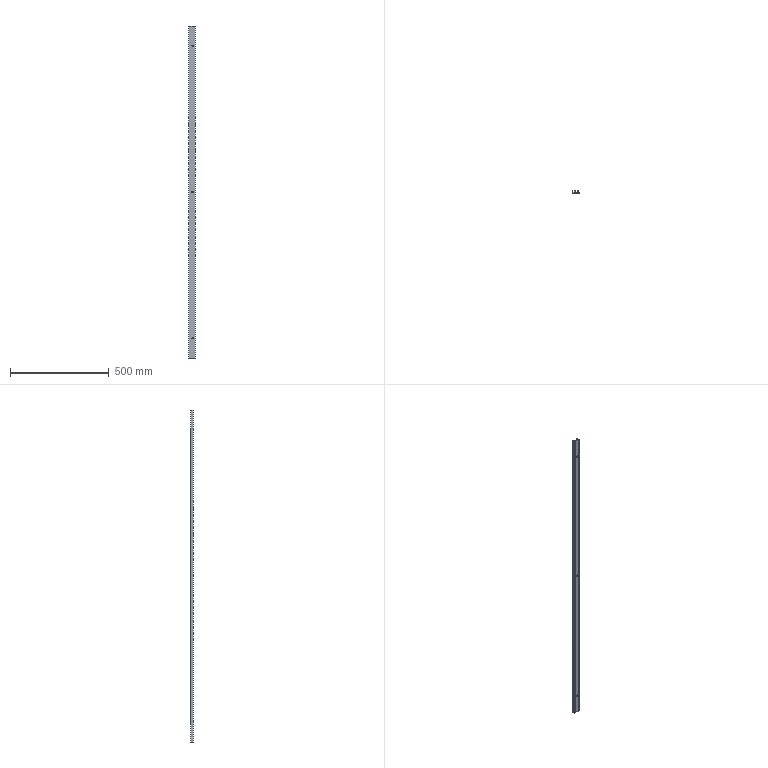Part | 1 solid | 31 faces | box 33.5 x 13.5 x 1682 mm | volume 314894 mm3 | plane 16 | cylinder 9 | cone 6 | commonest cylinder face diameters 2 x3 13.44 x3 4 x2 1.5 x1
STEP:
#1=CARTESIAN_POINT('',(20.,0.,1485.72));
#2=VERTEX_POINT('',#1);
#3=CARTESIAN_POINT('',(20.,0.,1478.28));
#4=VERTEX_POINT('',#3);
#5=CARTESIAN_POINT('',(20.,0.,1482.));
#6=DIRECTION('',(0.,-1.,0.));
#7=DIRECTION('',(0.,0.,-1.));
#8=AXIS2_PLACEMENT_3D('',#5,#6,#7);
#9=CIRCLE('',#8,3.72);
#10=EDGE_CURVE('',#2,#4,#9,.T.);
#11=ORIENTED_EDGE('',*,*,#10,.T.);
#12=CARTESIAN_POINT('',(20.,3.,1475.28));
#13=VERTEX_POINT('',#12);
#14=CARTESIAN_POINT('',(20.,3.,1475.28));
#15=DIRECTION('',(0.,0.7071,-0.7071));
#16=VECTOR('',#15,1000.);
#17=LINE('',#14,#16);
#18=EDGE_CURVE('',#4,#13,#17,.T.);
#19=ORIENTED_EDGE('',*,*,#18,.T.);
#20=CARTESIAN_POINT('',(20.,3.,1488.72));
#21=VERTEX_POINT('',#20);
#22=CARTESIAN_POINT('',(20.,3.,1482.));
#23=DIRECTION('',(0.,1.,0.));
#24=DIRECTION('',(0.,0.,1.));
#25=AXIS2_PLACEMENT_3D('',#22,#23,#24);
#26=CIRCLE('',#25,6.72);
#27=EDGE_CURVE('',#13,#21,#26,.T.);
#28=ORIENTED_EDGE('',*,*,#27,.T.);
#29=CARTESIAN_POINT('',(20.,3.,1488.72));
#30=DIRECTION('',(0.,0.7071,0.7071));
#31=VECTOR('',#30,1000.);
#32=LINE('',#29,#31);
#33=EDGE_CURVE('',#2,#21,#32,.T.);
#34=ORIENTED_EDGE('',*,*,#33,.F.);
#35=EDGE_LOOP('',(#11,#19,#28,#34));
#36=FACE_OUTER_BOUND('',#35,.T.);
#37=CARTESIAN_POINT('',(20.,3.,1482.));
#38=DIRECTION('',(0.,1.,0.));
#39=DIRECTION('',(0.,0.,1.));
#40=AXIS2_PLACEMENT_3D('',#37,#38,#39);
#41=CONICAL_SURFACE('',#40,6.72,0.7854);
#42=ADVANCED_FACE('',(#36),#41,.F.);
#43=CARTESIAN_POINT('',(20.,0.,3.72));
#44=VERTEX_POINT('',#43);
#45=CARTESIAN_POINT('',(20.,0.,-3.72));
#46=VERTEX_POINT('',#45);
#47=CARTESIAN_POINT('',(20.,0.,0.));
#48=DIRECTION('',(0.,-1.,0.));
#49=DIRECTION('',(0.,0.,-1.));
#50=AXIS2_PLACEMENT_3D('',#47,#48,#49);
#51=CIRCLE('',#50,3.72);
#52=EDGE_CURVE('',#44,#46,#51,.T.);
#53=ORIENTED_EDGE('',*,*,#52,.T.);
#54=CARTESIAN_POINT('',(20.,3.,-6.72));
#55=VERTEX_POINT('',#54);
#56=CARTESIAN_POINT('',(20.,3.,-6.72));
#57=DIRECTION('',(0.,0.7071,-0.7071));
#58=VECTOR('',#57,1000.);
#59=LINE('',#56,#58);
#60=EDGE_CURVE('',#46,#55,#59,.T.);
#61=ORIENTED_EDGE('',*,*,#60,.T.);
#62=CARTESIAN_POINT('',(20.,3.,6.72));
#63=VERTEX_POINT('',#62);
#64=CARTESIAN_POINT('',(20.,3.,0.));
#65=DIRECTION('',(0.,1.,0.));
#66=DIRECTION('',(0.,0.,1.));
#67=AXIS2_PLACEMENT_3D('',#64,#65,#66);
#68=CIRCLE('',#67,6.72);
#69=EDGE_CURVE('',#55,#63,#68,.T.);
#70=ORIENTED_EDGE('',*,*,#69,.T.);
#71=CARTESIAN_POINT('',(20.,3.,6.72));
#72=DIRECTION('',(0.,0.7071,0.7071));
#73=VECTOR('',#72,1000.);
#74=LINE('',#71,#73);
#75=EDGE_CURVE('',#44,#63,#74,.T.);
#76=ORIENTED_EDGE('',*,*,#75,.F.);
#77=EDGE_LOOP('',(#53,#61,#70,#76));
#78=FACE_OUTER_BOUND('',#77,.T.);
#79=CARTESIAN_POINT('',(20.,3.,0.));
#80=DIRECTION('',(0.,1.,0.));
#81=DIRECTION('',(0.,0.,1.));
#82=AXIS2_PLACEMENT_3D('',#79,#80,#81);
#83=CONICAL_SURFACE('',#82,6.72,0.7854);
#84=ADVANCED_FACE('',(#78),#83,.F.);
#85=CARTESIAN_POINT('',(20.,0.,744.72));
#86=VERTEX_POINT('',#85);
#87=CARTESIAN_POINT('',(20.,0.,737.28));
#88=VERTEX_POINT('',#87);
#89=CARTESIAN_POINT('',(20.,0.,741.));
#90=DIRECTION('',(0.,-1.,0.));
#91=DIRECTION('',(0.,0.,-1.));
#92=AXIS2_PLACEMENT_3D('',#89,#90,#91);
#93=CIRCLE('',#92,3.72);
#94=EDGE_CURVE('',#86,#88,#93,.T.);
#95=ORIENTED_EDGE('',*,*,#94,.T.);
#96=CARTESIAN_POINT('',(20.,3.,734.28));
#97=VERTEX_POINT('',#96);
#98=CARTESIAN_POINT('',(20.,3.,734.28));
#99=DIRECTION('',(0.,0.7071,-0.7071));
#100=VECTOR('',#99,1000.);
#101=LINE('',#98,#100);
#102=EDGE_CURVE('',#88,#97,#101,.T.);
#103=ORIENTED_EDGE('',*,*,#102,.T.);
#104=CARTESIAN_POINT('',(20.,3.,747.72));
#105=VERTEX_POINT('',#104);
#106=CARTESIAN_POINT('',(20.,3.,741.));
#107=DIRECTION('',(0.,1.,0.));
#108=DIRECTION('',(0.,0.,1.));
#109=AXIS2_PLACEMENT_3D('',#106,#107,#108);
#110=CIRCLE('',#109,6.72);
#111=EDGE_CURVE('',#97,#105,#110,.T.);
#112=ORIENTED_EDGE('',*,*,#111,.T.);
#113=CARTESIAN_POINT('',(20.,3.,747.72));
#114=DIRECTION('',(0.,0.7071,0.7071));
#115=VECTOR('',#114,1000.);
#116=LINE('',#113,#115);
#117=EDGE_CURVE('',#86,#105,#116,.T.);
#118=ORIENTED_EDGE('',*,*,#117,.F.);
#119=EDGE_LOOP('',(#95,#103,#112,#118));
#120=FACE_OUTER_BOUND('',#119,.T.);
#121=CARTESIAN_POINT('',(20.,3.,741.));
#122=DIRECTION('',(0.,1.,0.));
#123=DIRECTION('',(0.,0.,1.));
#124=AXIS2_PLACEMENT_3D('',#121,#122,#123);
#125=CONICAL_SURFACE('',#124,6.72,0.7854);
#126=ADVANCED_FACE('',(#120),#125,.F.);
#127=CARTESIAN_POINT('',(24.5,10.5,-4.991));
#128=VERTEX_POINT('',#127);
#129=CARTESIAN_POINT('',(24.5,10.5,-100.));
#130=VERTEX_POINT('',#129);
#131=CARTESIAN_POINT('',(24.5,10.5,-100.));
#132=DIRECTION('',(0.,0.,-1.));
#133=VECTOR('',#132,1000.);
#134=LINE('',#131,#133);
#135=EDGE_CURVE('',#128,#130,#134,.T.);
#136=ORIENTED_EDGE('',*,*,#135,.F.);
#137=CARTESIAN_POINT('',(24.5,10.5,4.991));
#138=VERTEX_POINT('',#137);
#139=CARTESIAN_POINT('',(24.5,10.5,-4.991));
#140=CARTESIAN_POINT('',(24.5,10.638,-4.991));
#141=CARTESIAN_POINT('',(24.515,10.777,-4.978));
#142=CARTESIAN_POINT('',(24.57,11.043,-4.927));
#143=CARTESIAN_POINT('',(24.611,11.171,-4.889));
#144=CARTESIAN_POINT('',(24.765,11.529,-4.74));
#145=CARTESIAN_POINT('',(24.907,11.728,-4.597));
#146=CARTESIAN_POINT('',(25.205,12.04,-4.256));
#147=CARTESIAN_POINT('',(25.365,12.156,-4.055));
#148=CARTESIAN_POINT('',(25.663,12.325,-3.627));
#149=CARTESIAN_POINT('',(25.806,12.38,-3.395));
#150=CARTESIAN_POINT('',(26.19,12.494,-2.672));
#151=CARTESIAN_POINT('',(26.387,12.501,-2.161));
#152=CARTESIAN_POINT('',(26.654,12.499,-1.091));
#153=CARTESIAN_POINT('',(26.72,12.488,-0.5481));
#154=CARTESIAN_POINT('',(26.72,12.488,0.2773));
#155=CARTESIAN_POINT('',(26.703,12.49,0.5529));
#156=CARTESIAN_POINT('',(26.636,12.496,1.095));
#157=CARTESIAN_POINT('',(26.586,12.499,1.362));
#158=CARTESIAN_POINT('',(26.388,12.501,2.155));
#159=CARTESIAN_POINT('',(26.188,12.493,2.677));
#160=CARTESIAN_POINT('',(25.805,12.38,3.396));
#161=CARTESIAN_POINT('',(25.662,12.324,3.629));
#162=CARTESIAN_POINT('',(25.438,12.197,3.95));
#163=CARTESIAN_POINT('',(25.362,12.147,4.053));
#164=CARTESIAN_POINT('',(25.208,12.03,4.249));
#165=CARTESIAN_POINT('',(25.13,11.961,4.342));
#166=CARTESIAN_POINT('',(24.98,11.805,4.513));
#167=CARTESIAN_POINT('',(24.908,11.717,4.591));
#168=CARTESIAN_POINT('',(24.774,11.518,4.73));
#169=CARTESIAN_POINT('',(24.714,11.408,4.79));
#170=CARTESIAN_POINT('',(24.612,11.172,4.888));
#171=CARTESIAN_POINT('',(24.57,11.043,4.927));
#172=CARTESIAN_POINT('',(24.515,10.778,4.978));
#173=CARTESIAN_POINT('',(24.5,10.64,4.991));
#174=CARTESIAN_POINT('',(24.5,10.5,4.991));
#175=B_SPLINE_CURVE_WITH_KNOTS('',3,(#139,#140,#141,#142,#143,#144,#145,#146,#147,#148,#149,#150,#151,#152,#153,#154,#155,#156,#157,#158,#159,#160,#161,#162,#163,#164,#165,#166,#167,#168,#169,#170,#171,#172,#173,#174),.UNSPECIFIED.,.F.,.F.,(4,2,2,2,2,2,2,2,2,2,2,2,2,2,2,2,2,4),(0.01321,0.01362,0.01403,0.01486,0.01569,0.01651,0.01816,0.01981,0.02064,0.02146,0.02311,0.02394,0.02435,0.02477,0.02518,0.02559,0.026,0.02642),.UNSPECIFIED.);
#176=EDGE_CURVE('',#128,#138,#175,.T.);
#177=ORIENTED_EDGE('',*,*,#176,.T.);
#178=CARTESIAN_POINT('',(24.5,10.5,736.009));
#179=VERTEX_POINT('',#178);
#180=CARTESIAN_POINT('',(24.5,10.5,-100.));
#181=DIRECTION('',(0.,0.,-1.));
#182=VECTOR('',#181,1000.);
#183=LINE('',#180,#182);
#184=EDGE_CURVE('',#179,#138,#183,.T.);
#185=ORIENTED_EDGE('',*,*,#184,.F.);
#186=CARTESIAN_POINT('',(24.5,10.5,745.991));
#187=VERTEX_POINT('',#186);
#188=CARTESIAN_POINT('',(24.5,10.5,736.009));
#189=CARTESIAN_POINT('',(24.5,10.638,736.009));
#190=CARTESIAN_POINT('',(24.515,10.777,736.022));
#191=CARTESIAN_POINT('',(24.57,11.043,736.073));
#192=CARTESIAN_POINT('',(24.611,11.171,736.111));
#193=CARTESIAN_POINT('',(24.765,11.529,736.26));
#194=CARTESIAN_POINT('',(24.907,11.728,736.403));
#195=CARTESIAN_POINT('',(25.205,12.04,736.744));
#196=CARTESIAN_POINT('',(25.365,12.156,736.945));
#197=CARTESIAN_POINT('',(25.663,12.325,737.373));
#198=CARTESIAN_POINT('',(25.806,12.38,737.605));
#199=CARTESIAN_POINT('',(26.19,12.494,738.328));
#200=CARTESIAN_POINT('',(26.387,12.501,738.839));
#201=CARTESIAN_POINT('',(26.654,12.499,739.909));
#202=CARTESIAN_POINT('',(26.72,12.488,740.452));
#203=CARTESIAN_POINT('',(26.72,12.488,741.277));
#204=CARTESIAN_POINT('',(26.703,12.49,741.553));
#205=CARTESIAN_POINT('',(26.636,12.496,742.095));
#206=CARTESIAN_POINT('',(26.586,12.499,742.362));
#207=CARTESIAN_POINT('',(26.388,12.501,743.155));
#208=CARTESIAN_POINT('',(26.188,12.493,743.677));
#209=CARTESIAN_POINT('',(25.805,12.38,744.396));
#210=CARTESIAN_POINT('',(25.662,12.324,744.629));
#211=CARTESIAN_POINT('',(25.438,12.197,744.95));
#212=CARTESIAN_POINT('',(25.362,12.147,745.053));
#213=CARTESIAN_POINT('',(25.208,12.03,745.249));
#214=CARTESIAN_POINT('',(25.13,11.961,745.342));
#215=CARTESIAN_POINT('',(24.98,11.805,745.513));
#216=CARTESIAN_POINT('',(24.908,11.717,745.591));
#217=CARTESIAN_POINT('',(24.774,11.518,745.73));
#218=CARTESIAN_POINT('',(24.714,11.408,745.79));
#219=CARTESIAN_POINT('',(24.612,11.172,745.888));
#220=CARTESIAN_POINT('',(24.57,11.043,745.927));
#221=CARTESIAN_POINT('',(24.515,10.778,745.978));
#222=CARTESIAN_POINT('',(24.5,10.64,745.991));
#223=CARTESIAN_POINT('',(24.5,10.5,745.991));
#224=B_SPLINE_CURVE_WITH_KNOTS('',3,(#188,#189,#190,#191,#192,#193,#194,#195,#196,#197,#198,#199,#200,#201,#202,#203,#204,#205,#206,#207,#208,#209,#210,#211,#212,#213,#214,#215,#216,#217,#218,#219,#220,#221,#222,#223),.UNSPECIFIED.,.F.,.F.,(4,2,2,2,2,2,2,2,2,2,2,2,2,2,2,2,2,4),(0.01321,0.01362,0.01403,0.01486,0.01569,0.01651,0.01816,0.01981,0.02064,0.02146,0.02311,0.02394,0.02435,0.02477,0.02518,0.02559,0.026,0.02642),.UNSPECIFIED.);
#225=EDGE_CURVE('',#179,#187,#224,.T.);
#226=ORIENTED_EDGE('',*,*,#225,.T.);
#227=CARTESIAN_POINT('',(24.5,10.5,1477.009));
#228=VERTEX_POINT('',#227);
#229=CARTESIAN_POINT('',(24.5,10.5,-100.));
#230=DIRECTION('',(0.,0.,-1.));
#231=VECTOR('',#230,1000.);
#232=LINE('',#229,#231);
#233=EDGE_CURVE('',#228,#187,#232,.T.);
#234=ORIENTED_EDGE('',*,*,#233,.F.);
#235=CARTESIAN_POINT('',(24.5,10.5,1486.991));
#236=VERTEX_POINT('',#235);
#237=CARTESIAN_POINT('',(24.5,10.5,1477.009));
#238=CARTESIAN_POINT('',(24.5,10.64,1477.009));
#239=CARTESIAN_POINT('',(24.514,10.776,1477.022));
#240=CARTESIAN_POINT('',(24.57,11.042,1477.073));
#241=CARTESIAN_POINT('',(24.611,11.171,1477.111));
#242=CARTESIAN_POINT('',(24.713,11.408,1477.209));
#243=CARTESIAN_POINT('',(24.775,11.519,1477.27));
#244=CARTESIAN_POINT('',(24.908,11.717,1477.409));
#245=CARTESIAN_POINT('',(24.981,11.806,1477.488));
#246=CARTESIAN_POINT('',(25.207,12.042,1477.746));
#247=CARTESIAN_POINT('',(25.363,12.155,1477.942));
#248=CARTESIAN_POINT('',(25.665,12.326,1478.376));
#249=CARTESIAN_POINT('',(25.806,12.38,1478.605));
#250=CARTESIAN_POINT('',(26.061,12.456,1479.084));
#251=CARTESIAN_POINT('',(26.176,12.476,1479.337));
#252=CARTESIAN_POINT('',(26.372,12.498,1479.849));
#253=CARTESIAN_POINT('',(26.454,12.501,1480.109));
#254=CARTESIAN_POINT('',(26.586,12.499,1480.638));
#255=CARTESIAN_POINT('',(26.636,12.496,1480.907));
#256=CARTESIAN_POINT('',(26.703,12.49,1481.453));
#257=CARTESIAN_POINT('',(26.72,12.488,1481.729));
#258=CARTESIAN_POINT('',(26.72,12.488,1482.275));
#259=CARTESIAN_POINT('',(26.703,12.49,1482.547));
#260=CARTESIAN_POINT('',(26.637,12.496,1483.089));
#261=CARTESIAN_POINT('',(26.587,12.499,1483.36));
#262=CARTESIAN_POINT('',(26.387,12.501,1484.161));
#263=CARTESIAN_POINT('',(26.191,12.494,1484.671));
#264=CARTESIAN_POINT('',(25.805,12.38,1485.396));
#265=CARTESIAN_POINT('',(25.663,12.325,1485.627));
#266=CARTESIAN_POINT('',(25.364,12.155,1486.057));
#267=CARTESIAN_POINT('',(25.205,12.039,1486.256));
#268=CARTESIAN_POINT('',(24.981,11.805,1486.512));
#269=CARTESIAN_POINT('',(24.907,11.716,1486.592));
#270=CARTESIAN_POINT('',(24.774,11.518,1486.73));
#271=CARTESIAN_POINT('',(24.714,11.409,1486.79));
#272=CARTESIAN_POINT('',(24.611,11.17,1486.889));
#273=CARTESIAN_POINT('',(24.571,11.044,1486.926));
#274=CARTESIAN_POINT('',(24.515,10.78,1486.977));
#275=CARTESIAN_POINT('',(24.5,10.64,1486.991));
#276=CARTESIAN_POINT('',(24.5,10.5,1486.991));
#277=B_SPLINE_CURVE_WITH_KNOTS('',3,(#237,#238,#239,#240,#241,#242,#243,#244,#245,#246,#247,#248,#249,#250,#251,#252,#253,#254,#255,#256,#257,#258,#259,#260,#261,#262,#263,#264,#265,#266,#267,#268,#269,#270,#271,#272,#273,#274,#275,#276),.UNSPECIFIED.,.F.,.F.,(4,2,2,2,2,2,2,2,2,2,2,2,2,2,2,2,2,2,2,4),(0.,0.0004127,0.0008255,0.001238,0.001651,0.002476,0.003302,0.004127,0.004953,0.005778,0.006604,0.007429,0.008255,0.009906,0.01073,0.01156,0.01197,0.01238,0.01279,0.01321),.UNSPECIFIED.);
#278=EDGE_CURVE('',#228,#236,#277,.T.);
#279=ORIENTED_EDGE('',*,*,#278,.T.);
#280=CARTESIAN_POINT('',(24.5,10.5,1582.));
#281=VERTEX_POINT('',#280);
#282=CARTESIAN_POINT('',(24.5,10.5,-100.));
#283=DIRECTION('',(0.,0.,-1.));
#284=VECTOR('',#283,1000.);
#285=LINE('',#282,#284);
#286=EDGE_CURVE('',#281,#236,#285,.T.);
#287=ORIENTED_EDGE('',*,*,#286,.F.);
#288=CARTESIAN_POINT('',(28.5,10.5,1582.));
#289=VERTEX_POINT('',#288);
#290=CARTESIAN_POINT('',(26.5,10.5,1582.));
#291=DIRECTION('',(0.,0.,1.));
#292=DIRECTION('',(1.,0.,0.));
#293=AXIS2_PLACEMENT_3D('',#290,#291,#292);
#294=CIRCLE('',#293,2.);
#295=EDGE_CURVE('',#289,#281,#294,.T.);
#296=ORIENTED_EDGE('',*,*,#295,.F.);
#297=CARTESIAN_POINT('',(28.5,10.5,-100.));
#298=VERTEX_POINT('',#297);
#299=CARTESIAN_POINT('',(28.5,10.5,-100.));
#300=DIRECTION('',(0.,0.,-1.));
#301=VECTOR('',#300,1000.);
#302=LINE('',#299,#301);
#303=EDGE_CURVE('',#289,#298,#302,.T.);
#304=ORIENTED_EDGE('',*,*,#303,.T.);
#305=CARTESIAN_POINT('',(26.5,10.5,-100.));
#306=DIRECTION('',(0.,0.,1.));
#307=DIRECTION('',(-1.,0.,0.));
#308=AXIS2_PLACEMENT_3D('',#305,#306,#307);
#309=CIRCLE('',#308,2.);
#310=EDGE_CURVE('',#298,#130,#309,.T.);
#311=ORIENTED_EDGE('',*,*,#310,.T.);
#312=EDGE_LOOP('',(#136,#177,#185,#226,#234,#279,#287,#296,#304,#311));
#313=FACE_OUTER_BOUND('',#312,.T.);
#314=CARTESIAN_POINT('',(26.5,10.5,-100.));
#315=DIRECTION('',(0.,0.,-1.));
#316=DIRECTION('',(-1.,0.,0.));
#317=AXIS2_PLACEMENT_3D('',#314,#315,#316);
#318=CYLINDRICAL_SURFACE('',#317,2.);
#319=ADVANCED_FACE('',(#313),#318,.T.);
#320=CARTESIAN_POINT('',(24.5,3.,-4.991));
#321=VERTEX_POINT('',#320);
#322=CARTESIAN_POINT('',(24.5,3.,-100.));
#323=VERTEX_POINT('',#322);
#324=CARTESIAN_POINT('',(24.5,3.,-100.));
#325=DIRECTION('',(0.,0.,-1.));
#326=VECTOR('',#325,1000.);
#327=LINE('',#324,#326);
#328=EDGE_CURVE('',#321,#323,#327,.T.);
#329=ORIENTED_EDGE('',*,*,#328,.F.);
#330=CARTESIAN_POINT('',(24.5,13.5,-4.991));
#331=DIRECTION('',(0.,1.,0.));
#332=VECTOR('',#331,1000.);
#333=LINE('',#330,#332);
#334=EDGE_CURVE('',#321,#128,#333,.T.);
#335=ORIENTED_EDGE('',*,*,#334,.T.);
#336=ORIENTED_EDGE('',*,*,#135,.T.);
#337=CARTESIAN_POINT('',(24.5,1.,-100.));
#338=DIRECTION('',(0.,-1.,0.));
#339=VECTOR('',#338,1000.);
#340=LINE('',#337,#339);
#341=EDGE_CURVE('',#130,#323,#340,.T.);
#342=ORIENTED_EDGE('',*,*,#341,.T.);
#343=EDGE_LOOP('',(#329,#335,#336,#342));
#344=FACE_OUTER_BOUND('',#343,.T.);
#345=CARTESIAN_POINT('',(24.5,10.5,-100.));
#346=DIRECTION('',(-1.,0.,0.));
#347=DIRECTION('',(0.,0.,1.));
#348=AXIS2_PLACEMENT_3D('',#345,#346,#347);
#349=PLANE('',#348);
#350=ADVANCED_FACE('',(#344),#349,.T.);
#351=ORIENTED_EDGE('',*,*,#184,.T.);
#352=CARTESIAN_POINT('',(24.5,3.,4.991));
#353=VERTEX_POINT('',#352);
#354=CARTESIAN_POINT('',(24.5,13.5,4.991));
#355=DIRECTION('',(0.,-1.,0.));
#356=VECTOR('',#355,1000.);
#357=LINE('',#354,#356);
#358=EDGE_CURVE('',#138,#353,#357,.T.);
#359=ORIENTED_EDGE('',*,*,#358,.T.);
#360=CARTESIAN_POINT('',(24.5,3.,736.009));
#361=VERTEX_POINT('',#360);
#362=CARTESIAN_POINT('',(24.5,3.,-100.));
#363=DIRECTION('',(0.,0.,-1.));
#364=VECTOR('',#363,1000.);
#365=LINE('',#362,#364);
#366=EDGE_CURVE('',#361,#353,#365,.T.);
#367=ORIENTED_EDGE('',*,*,#366,.F.);
#368=CARTESIAN_POINT('',(24.5,13.5,736.009));
#369=DIRECTION('',(0.,1.,0.));
#370=VECTOR('',#369,1000.);
#371=LINE('',#368,#370);
#372=EDGE_CURVE('',#361,#179,#371,.T.);
#373=ORIENTED_EDGE('',*,*,#372,.T.);
#374=EDGE_LOOP('',(#351,#359,#367,#373));
#375=FACE_OUTER_BOUND('',#374,.T.);
#376=CARTESIAN_POINT('',(24.5,10.5,-100.));
#377=DIRECTION('',(-1.,0.,0.));
#378=DIRECTION('',(0.,0.,1.));
#379=AXIS2_PLACEMENT_3D('',#376,#377,#378);
#380=PLANE('',#379);
#381=ADVANCED_FACE('',(#375),#380,.T.);
#382=ORIENTED_EDGE('',*,*,#233,.T.);
#383=CARTESIAN_POINT('',(24.5,3.,745.991));
#384=VERTEX_POINT('',#383);
#385=CARTESIAN_POINT('',(24.5,13.5,745.991));
#386=DIRECTION('',(0.,-1.,0.));
#387=VECTOR('',#386,1000.);
#388=LINE('',#385,#387);
#389=EDGE_CURVE('',#187,#384,#388,.T.);
#390=ORIENTED_EDGE('',*,*,#389,.T.);
#391=CARTESIAN_POINT('',(24.5,3.,1477.009));
#392=VERTEX_POINT('',#391);
#393=CARTESIAN_POINT('',(24.5,3.,-100.));
#394=DIRECTION('',(0.,0.,-1.));
#395=VECTOR('',#394,1000.);
#396=LINE('',#393,#395);
#397=EDGE_CURVE('',#392,#384,#396,.T.);
#398=ORIENTED_EDGE('',*,*,#397,.F.);
#399=CARTESIAN_POINT('',(24.5,13.5,1477.009));
#400=DIRECTION('',(0.,1.,0.));
#401=VECTOR('',#400,1000.);
#402=LINE('',#399,#401);
#403=EDGE_CURVE('',#392,#228,#402,.T.);
#404=ORIENTED_EDGE('',*,*,#403,.T.);
#405=EDGE_LOOP('',(#382,#390,#398,#404));
#406=FACE_OUTER_BOUND('',#405,.T.);
#407=CARTESIAN_POINT('',(24.5,10.5,-100.));
#408=DIRECTION('',(-1.,0.,0.));
#409=DIRECTION('',(0.,0.,1.));
#410=AXIS2_PLACEMENT_3D('',#407,#408,#409);
#411=PLANE('',#410);
#412=ADVANCED_FACE('',(#406),#411,.T.);
#413=ORIENTED_EDGE('',*,*,#286,.T.);
#414=CARTESIAN_POINT('',(24.5,3.,1486.991));
#415=VERTEX_POINT('',#414);
#416=CARTESIAN_POINT('',(24.5,13.5,1486.991));
#417=DIRECTION('',(0.,-1.,0.));
#418=VECTOR('',#417,1000.);
#419=LINE('',#416,#418);
#420=EDGE_CURVE('',#236,#415,#419,.T.);
#421=ORIENTED_EDGE('',*,*,#420,.T.);
#422=CARTESIAN_POINT('',(24.5,3.,1582.));
#423=VERTEX_POINT('',#422);
#424=CARTESIAN_POINT('',(24.5,3.,-100.));
#425=DIRECTION('',(0.,0.,-1.));
#426=VECTOR('',#425,1000.);
#427=LINE('',#424,#426);
#428=EDGE_CURVE('',#423,#415,#427,.T.);
#429=ORIENTED_EDGE('',*,*,#428,.F.);
#430=CARTESIAN_POINT('',(24.5,1.,1582.));
#431=DIRECTION('',(0.,-1.,0.));
#432=VECTOR('',#431,1000.);
#433=LINE('',#430,#432);
#434=EDGE_CURVE('',#281,#423,#433,.T.);
#435=ORIENTED_EDGE('',*,*,#434,.F.);
#436=EDGE_LOOP('',(#413,#421,#429,#435));
#437=FACE_OUTER_BOUND('',#436,.T.);
#438=CARTESIAN_POINT('',(24.5,10.5,-100.));
#439=DIRECTION('',(-1.,0.,0.));
#440=DIRECTION('',(0.,0.,1.));
#441=AXIS2_PLACEMENT_3D('',#438,#439,#440);
#442=PLANE('',#441);
#443=ADVANCED_FACE('',(#437),#442,.T.);
#444=ORIENTED_EDGE('',*,*,#10,.F.);
#445=CARTESIAN_POINT('',(20.,0.,1482.));
#446=DIRECTION('',(0.,-1.,0.));
#447=DIRECTION('',(0.,0.,-1.));
#448=AXIS2_PLACEMENT_3D('',#445,#446,#447);
#449=CIRCLE('',#448,3.72);
#450=EDGE_CURVE('',#4,#2,#449,.T.);
#451=ORIENTED_EDGE('',*,*,#450,.F.);
#452=EDGE_LOOP('',(#444,#451));
#453=FACE_BOUND('',#452,.T.);
#454=ORIENTED_EDGE('',*,*,#52,.F.);
#455=CARTESIAN_POINT('',(20.,0.,0.));
#456=DIRECTION('',(0.,-1.,0.));
#457=DIRECTION('',(0.,0.,-1.));
#458=AXIS2_PLACEMENT_3D('',#455,#456,#457);
#459=CIRCLE('',#458,3.72);
#460=EDGE_CURVE('',#46,#44,#459,.T.);
#461=ORIENTED_EDGE('',*,*,#460,.F.);
#462=EDGE_LOOP('',(#454,#461));
#463=FACE_BOUND('',#462,.T.);
#464=CARTESIAN_POINT('',(1.,0.,-100.));
#465=VERTEX_POINT('',#464);
#466=CARTESIAN_POINT('',(32.5,0.,-100.));
#467=VERTEX_POINT('',#466);
#468=CARTESIAN_POINT('',(1.,0.,-100.));
#469=DIRECTION('',(1.,0.,0.));
#470=VECTOR('',#469,1000.);
#471=LINE('',#468,#470);
#472=EDGE_CURVE('',#465,#467,#471,.T.);
#473=ORIENTED_EDGE('',*,*,#472,.T.);
#474=CARTESIAN_POINT('',(32.5,0.,1582.));
#475=VERTEX_POINT('',#474);
#476=CARTESIAN_POINT('',(32.5,0.,-100.));
#477=DIRECTION('',(0.,0.,1.));
#478=VECTOR('',#477,1000.);
#479=LINE('',#476,#478);
#480=EDGE_CURVE('',#467,#475,#479,.T.);
#481=ORIENTED_EDGE('',*,*,#480,.T.);
#482=CARTESIAN_POINT('',(1.,0.,1582.));
#483=VERTEX_POINT('',#482);
#484=CARTESIAN_POINT('',(1.,0.,1582.));
#485=DIRECTION('',(-1.,0.,0.));
#486=VECTOR('',#485,1000.);
#487=LINE('',#484,#486);
#488=EDGE_CURVE('',#475,#483,#487,.T.);
#489=ORIENTED_EDGE('',*,*,#488,.T.);
#490=CARTESIAN_POINT('',(1.,0.,-100.));
#491=DIRECTION('',(0.,0.,-1.));
#492=VECTOR('',#491,1000.);
#493=LINE('',#490,#492);
#494=EDGE_CURVE('',#483,#465,#493,.T.);
#495=ORIENTED_EDGE('',*,*,#494,.T.);
#496=EDGE_LOOP('',(#473,#481,#489,#495));
#497=FACE_OUTER_BOUND('',#496,.T.);
#498=ORIENTED_EDGE('',*,*,#94,.F.);
#499=CARTESIAN_POINT('',(20.,0.,741.));
#500=DIRECTION('',(0.,-1.,0.));
#501=DIRECTION('',(0.,0.,-1.));
#502=AXIS2_PLACEMENT_3D('',#499,#500,#501);
#503=CIRCLE('',#502,3.72);
#504=EDGE_CURVE('',#88,#86,#503,.T.);
#505=ORIENTED_EDGE('',*,*,#504,.F.);
#506=EDGE_LOOP('',(#498,#505));
#507=FACE_BOUND('',#506,.T.);
#508=CARTESIAN_POINT('',(1.,0.,-100.));
#509=DIRECTION('',(0.,-1.,0.));
#510=DIRECTION('',(0.,0.,-1.));
#511=AXIS2_PLACEMENT_3D('',#508,#509,#510);
#512=PLANE('',#511);
#513=ADVANCED_FACE('',(#453,#463,#497,#507),#512,.T.);
#514=CARTESIAN_POINT('',(33.5,1.,-100.));
#515=VERTEX_POINT('',#514);
#516=CARTESIAN_POINT('',(32.5,1.,-100.));
#517=DIRECTION('',(0.,0.,1.));
#518=DIRECTION('',(-1.,0.,0.));
#519=AXIS2_PLACEMENT_3D('',#516,#517,#518);
#520=CIRCLE('',#519,1.);
#521=EDGE_CURVE('',#467,#515,#520,.T.);
#522=ORIENTED_EDGE('',*,*,#521,.T.);
#523=CARTESIAN_POINT('',(33.5,1.,1582.));
#524=VERTEX_POINT('',#523);
#525=CARTESIAN_POINT('',(33.5,1.,-100.));
#526=DIRECTION('',(0.,0.,1.));
#527=VECTOR('',#526,1000.);
#528=LINE('',#525,#527);
#529=EDGE_CURVE('',#515,#524,#528,.T.);
#530=ORIENTED_EDGE('',*,*,#529,.T.);
#531=CARTESIAN_POINT('',(32.5,1.,1582.));
#532=DIRECTION('',(0.,0.,-1.));
#533=DIRECTION('',(1.,0.,0.));
#534=AXIS2_PLACEMENT_3D('',#531,#532,#533);
#535=CIRCLE('',#534,1.);
#536=EDGE_CURVE('',#524,#475,#535,.T.);
#537=ORIENTED_EDGE('',*,*,#536,.T.);
#538=ORIENTED_EDGE('',*,*,#480,.F.);
#539=EDGE_LOOP('',(#522,#530,#537,#538));
#540=FACE_OUTER_BOUND('',#539,.T.);
#541=CARTESIAN_POINT('',(32.5,1.,-100.));
#542=DIRECTION('',(0.,0.,-1.));
#543=DIRECTION('',(-1.,0.,0.));
#544=AXIS2_PLACEMENT_3D('',#541,#542,#543);
#545=CYLINDRICAL_SURFACE('',#544,1.);
#546=ADVANCED_FACE('',(#540),#545,.T.);
#547=CARTESIAN_POINT('',(1.5,12.75,-100.));
#548=VERTEX_POINT('',#547);
#549=CARTESIAN_POINT('',(0.,12.75,-100.));
#550=VERTEX_POINT('',#549);
#551=CARTESIAN_POINT('',(0.75,12.75,-100.));
#552=DIRECTION('',(0.,0.,1.));
#553=DIRECTION('',(-1.,0.,0.));
#554=AXIS2_PLACEMENT_3D('',#551,#552,#553);
#555=CIRCLE('',#554,0.75);
#556=EDGE_CURVE('',#548,#550,#555,.T.);
#557=ORIENTED_EDGE('',*,*,#556,.F.);
#558=CARTESIAN_POINT('',(1.5,3.,-100.));
#559=VERTEX_POINT('',#558);
#560=CARTESIAN_POINT('',(1.5,1.,-100.));
#561=DIRECTION('',(0.,1.,0.));
#562=VECTOR('',#561,1000.);
#563=LINE('',#560,#562);
#564=EDGE_CURVE('',#559,#548,#563,.T.);
#565=ORIENTED_EDGE('',*,*,#564,.F.);
#566=CARTESIAN_POINT('',(8.5,3.,-100.));
#567=VERTEX_POINT('',#566);
#568=CARTESIAN_POINT('',(1.,3.,-100.));
#569=DIRECTION('',(-1.,0.,0.));
#570=VECTOR('',#569,1000.);
#571=LINE('',#568,#570);
#572=EDGE_CURVE('',#567,#559,#571,.T.);
#573=ORIENTED_EDGE('',*,*,#572,.F.);
#574=CARTESIAN_POINT('',(8.5,10.5,-100.));
#575=VERTEX_POINT('',#574);
#576=CARTESIAN_POINT('',(8.5,1.,-100.));
#577=DIRECTION('',(0.,-1.,0.));
#578=VECTOR('',#577,1000.);
#579=LINE('',#576,#578);
#580=EDGE_CURVE('',#575,#567,#579,.T.);
#581=ORIENTED_EDGE('',*,*,#580,.F.);
#582=CARTESIAN_POINT('',(12.5,10.5,-100.));
#583=VERTEX_POINT('',#582);
#584=CARTESIAN_POINT('',(10.5,10.5,-100.));
#585=DIRECTION('',(0.,0.,1.));
#586=DIRECTION('',(-1.,0.,0.));
#587=AXIS2_PLACEMENT_3D('',#584,#585,#586);
#588=CIRCLE('',#587,2.);
#589=EDGE_CURVE('',#583,#575,#588,.T.);
#590=ORIENTED_EDGE('',*,*,#589,.F.);
#591=CARTESIAN_POINT('',(12.5,3.,-100.));
#592=VERTEX_POINT('',#591);
#593=CARTESIAN_POINT('',(12.5,1.,-100.));
#594=DIRECTION('',(0.,1.,0.));
#595=VECTOR('',#594,1000.);
#596=LINE('',#593,#595);
#597=EDGE_CURVE('',#592,#583,#596,.T.);
#598=ORIENTED_EDGE('',*,*,#597,.F.);
#599=CARTESIAN_POINT('',(1.,3.,-100.));
#600=DIRECTION('',(-1.,0.,0.));
#601=VECTOR('',#600,1000.);
#602=LINE('',#599,#601);
#603=EDGE_CURVE('',#323,#592,#602,.T.);
#604=ORIENTED_EDGE('',*,*,#603,.F.);
#605=ORIENTED_EDGE('',*,*,#341,.F.);
#606=ORIENTED_EDGE('',*,*,#310,.F.);
#607=CARTESIAN_POINT('',(28.5,3.,-100.));
#608=VERTEX_POINT('',#607);
#609=CARTESIAN_POINT('',(28.5,1.,-100.));
#610=DIRECTION('',(0.,1.,0.));
#611=VECTOR('',#610,1000.);
#612=LINE('',#609,#611);
#613=EDGE_CURVE('',#608,#298,#612,.T.);
#614=ORIENTED_EDGE('',*,*,#613,.F.);
#615=CARTESIAN_POINT('',(32.5,3.,-100.));
#616=VERTEX_POINT('',#615);
#617=CARTESIAN_POINT('',(1.,3.,-100.));
#618=DIRECTION('',(-1.,0.,0.));
#619=VECTOR('',#618,1000.);
#620=LINE('',#617,#619);
#621=EDGE_CURVE('',#616,#608,#620,.T.);
#622=ORIENTED_EDGE('',*,*,#621,.F.);
#623=CARTESIAN_POINT('',(33.5,2.,-100.));
#624=VERTEX_POINT('',#623);
#625=CARTESIAN_POINT('',(32.5,2.,-100.));
#626=DIRECTION('',(0.,0.,1.));
#627=DIRECTION('',(-1.,0.,0.));
#628=AXIS2_PLACEMENT_3D('',#625,#626,#627);
#629=CIRCLE('',#628,1.);
#630=EDGE_CURVE('',#624,#616,#629,.T.);
#631=ORIENTED_EDGE('',*,*,#630,.F.);
#632=CARTESIAN_POINT('',(33.5,1.,-100.));
#633=DIRECTION('',(0.,1.,0.));
#634=VECTOR('',#633,1000.);
#635=LINE('',#632,#634);
#636=EDGE_CURVE('',#515,#624,#635,.T.);
#637=ORIENTED_EDGE('',*,*,#636,.F.);
#638=ORIENTED_EDGE('',*,*,#521,.F.);
#639=ORIENTED_EDGE('',*,*,#472,.F.);
#640=CARTESIAN_POINT('',(0.,1.,-100.));
#641=VERTEX_POINT('',#640);
#642=CARTESIAN_POINT('',(1.,1.,-100.));
#643=DIRECTION('',(0.,0.,1.));
#644=DIRECTION('',(-1.,0.,0.));
#645=AXIS2_PLACEMENT_3D('',#642,#643,#644);
#646=CIRCLE('',#645,1.);
#647=EDGE_CURVE('',#641,#465,#646,.T.);
#648=ORIENTED_EDGE('',*,*,#647,.F.);
#649=CARTESIAN_POINT('',(0.,1.,-100.));
#650=DIRECTION('',(0.,-1.,0.));
#651=VECTOR('',#650,1000.);
#652=LINE('',#649,#651);
#653=EDGE_CURVE('',#550,#641,#652,.T.);
#654=ORIENTED_EDGE('',*,*,#653,.F.);
#655=EDGE_LOOP('',(#557,#565,#573,#581,#590,#598,#604,#605,#606,#614,#622,#631,#637,#638,#639,#648,#654));
#656=FACE_OUTER_BOUND('',#655,.T.);
#657=CARTESIAN_POINT('',(1.,1.,-100.));
#658=DIRECTION('',(0.,0.,1.));
#659=DIRECTION('',(1.,0.,0.));
#660=AXIS2_PLACEMENT_3D('',#657,#658,#659);
#661=PLANE('',#660);
#662=ADVANCED_FACE('',(#656),#661,.F.);
#663=ORIENTED_EDGE('',*,*,#647,.T.);
#664=ORIENTED_EDGE('',*,*,#494,.F.);
#665=CARTESIAN_POINT('',(0.,1.,1582.));
#666=VERTEX_POINT('',#665);
#667=CARTESIAN_POINT('',(1.,1.,1582.));
#668=DIRECTION('',(0.,0.,-1.));
#669=DIRECTION('',(1.,0.,0.));
#670=AXIS2_PLACEMENT_3D('',#667,#668,#669);
#671=CIRCLE('',#670,1.);
#672=EDGE_CURVE('',#483,#666,#671,.T.);
#673=ORIENTED_EDGE('',*,*,#672,.T.);
#674=CARTESIAN_POINT('',(0.,1.,-100.));
#675=DIRECTION('',(0.,0.,-1.));
#676=VECTOR('',#675,1000.);
#677=LINE('',#674,#676);
#678=EDGE_CURVE('',#666,#641,#677,.T.);
#679=ORIENTED_EDGE('',*,*,#678,.T.);
#680=EDGE_LOOP('',(#663,#664,#673,#679));
#681=FACE_OUTER_BOUND('',#680,.T.);
#682=CARTESIAN_POINT('',(1.,1.,-100.));
#683=DIRECTION('',(0.,0.,-1.));
#684=DIRECTION('',(-1.,0.,0.));
#685=AXIS2_PLACEMENT_3D('',#682,#683,#684);
#686=CYLINDRICAL_SURFACE('',#685,1.);
#687=ADVANCED_FACE('',(#681),#686,.T.);
#688=CARTESIAN_POINT('',(1.5,3.,1582.));
#689=VERTEX_POINT('',#688);
#690=CARTESIAN_POINT('',(1.5,12.75,1582.));
#691=VERTEX_POINT('',#690);
#692=CARTESIAN_POINT('',(1.5,1.,1582.));
#693=DIRECTION('',(0.,1.,0.));
#694=VECTOR('',#693,1000.);
#695=LINE('',#692,#694);
#696=EDGE_CURVE('',#689,#691,#695,.T.);
#697=ORIENTED_EDGE('',*,*,#696,.T.);
#698=CARTESIAN_POINT('',(0.,12.75,1582.));
#699=VERTEX_POINT('',#698);
#700=CARTESIAN_POINT('',(0.75,12.75,1582.));
#701=DIRECTION('',(0.,0.,1.));
#702=DIRECTION('',(1.,0.,0.));
#703=AXIS2_PLACEMENT_3D('',#700,#701,#702);
#704=CIRCLE('',#703,0.75);
#705=EDGE_CURVE('',#691,#699,#704,.T.);
#706=ORIENTED_EDGE('',*,*,#705,.T.);
#707=CARTESIAN_POINT('',(0.,1.,1582.));
#708=DIRECTION('',(0.,-1.,0.));
#709=VECTOR('',#708,1000.);
#710=LINE('',#707,#709);
#711=EDGE_CURVE('',#699,#666,#710,.T.);
#712=ORIENTED_EDGE('',*,*,#711,.T.);
#713=ORIENTED_EDGE('',*,*,#672,.F.);
#714=ORIENTED_EDGE('',*,*,#488,.F.);
#715=ORIENTED_EDGE('',*,*,#536,.F.);
#716=CARTESIAN_POINT('',(33.5,2.,1582.));
#717=VERTEX_POINT('',#716);
#718=CARTESIAN_POINT('',(33.5,1.,1582.));
#719=DIRECTION('',(0.,1.,0.));
#720=VECTOR('',#719,1000.);
#721=LINE('',#718,#720);
#722=EDGE_CURVE('',#524,#717,#721,.T.);
#723=ORIENTED_EDGE('',*,*,#722,.T.);
#724=CARTESIAN_POINT('',(32.5,3.,1582.));
#725=VERTEX_POINT('',#724);
#726=CARTESIAN_POINT('',(32.5,2.,1582.));
#727=DIRECTION('',(0.,0.,-1.));
#728=DIRECTION('',(1.,0.,0.));
#729=AXIS2_PLACEMENT_3D('',#726,#727,#728);
#730=CIRCLE('',#729,1.);
#731=EDGE_CURVE('',#725,#717,#730,.T.);
#732=ORIENTED_EDGE('',*,*,#731,.F.);
#733=CARTESIAN_POINT('',(28.5,3.,1582.));
#734=VERTEX_POINT('',#733);
#735=CARTESIAN_POINT('',(1.,3.,1582.));
#736=DIRECTION('',(-1.,0.,0.));
#737=VECTOR('',#736,1000.);
#738=LINE('',#735,#737);
#739=EDGE_CURVE('',#725,#734,#738,.T.);
#740=ORIENTED_EDGE('',*,*,#739,.T.);
#741=CARTESIAN_POINT('',(28.5,1.,1582.));
#742=DIRECTION('',(0.,1.,0.));
#743=VECTOR('',#742,1000.);
#744=LINE('',#741,#743);
#745=EDGE_CURVE('',#734,#289,#744,.T.);
#746=ORIENTED_EDGE('',*,*,#745,.T.);
#747=ORIENTED_EDGE('',*,*,#295,.T.);
#748=ORIENTED_EDGE('',*,*,#434,.T.);
#749=CARTESIAN_POINT('',(12.5,3.,1582.));
#750=VERTEX_POINT('',#749);
#751=CARTESIAN_POINT('',(1.,3.,1582.));
#752=DIRECTION('',(-1.,0.,0.));
#753=VECTOR('',#752,1000.);
#754=LINE('',#751,#753);
#755=EDGE_CURVE('',#423,#750,#754,.T.);
#756=ORIENTED_EDGE('',*,*,#755,.T.);
#757=CARTESIAN_POINT('',(12.5,10.5,1582.));
#758=VERTEX_POINT('',#757);
#759=CARTESIAN_POINT('',(12.5,1.,1582.));
#760=DIRECTION('',(0.,1.,0.));
#761=VECTOR('',#760,1000.);
#762=LINE('',#759,#761);
#763=EDGE_CURVE('',#750,#758,#762,.T.);
#764=ORIENTED_EDGE('',*,*,#763,.T.);
#765=CARTESIAN_POINT('',(8.5,10.5,1582.));
#766=VERTEX_POINT('',#765);
#767=CARTESIAN_POINT('',(10.5,10.5,1582.));
#768=DIRECTION('',(0.,0.,1.));
#769=DIRECTION('',(1.,0.,0.));
#770=AXIS2_PLACEMENT_3D('',#767,#768,#769);
#771=CIRCLE('',#770,2.);
#772=EDGE_CURVE('',#758,#766,#771,.T.);
#773=ORIENTED_EDGE('',*,*,#772,.T.);
#774=CARTESIAN_POINT('',(8.5,3.,1582.));
#775=VERTEX_POINT('',#774);
#776=CARTESIAN_POINT('',(8.5,1.,1582.));
#777=DIRECTION('',(0.,-1.,0.));
#778=VECTOR('',#777,1000.);
#779=LINE('',#776,#778);
#780=EDGE_CURVE('',#766,#775,#779,.T.);
#781=ORIENTED_EDGE('',*,*,#780,.T.);
#782=CARTESIAN_POINT('',(1.,3.,1582.));
#783=DIRECTION('',(-1.,0.,0.));
#784=VECTOR('',#783,1000.);
#785=LINE('',#782,#784);
#786=EDGE_CURVE('',#775,#689,#785,.T.);
#787=ORIENTED_EDGE('',*,*,#786,.T.);
#788=EDGE_LOOP('',(#697,#706,#712,#713,#714,#715,#723,#732,#740,#746,#747,#748,#756,#764,#773,#781,#787));
#789=FACE_OUTER_BOUND('',#788,.T.);
#790=CARTESIAN_POINT('',(1.,1.,1582.));
#791=DIRECTION('',(0.,0.,1.));
#792=DIRECTION('',(1.,0.,0.));
#793=AXIS2_PLACEMENT_3D('',#790,#791,#792);
#794=PLANE('',#793);
#795=ADVANCED_FACE('',(#789),#794,.T.);
#796=ORIENTED_EDGE('',*,*,#636,.T.);
#797=CARTESIAN_POINT('',(33.5,2.,-100.));
#798=DIRECTION('',(0.,0.,1.));
#799=VECTOR('',#798,1000.);
#800=LINE('',#797,#799);
#801=EDGE_CURVE('',#624,#717,#800,.T.);
#802=ORIENTED_EDGE('',*,*,#801,.T.);
#803=ORIENTED_EDGE('',*,*,#722,.F.);
#804=ORIENTED_EDGE('',*,*,#529,.F.);
#805=EDGE_LOOP('',(#796,#802,#803,#804));
#806=FACE_OUTER_BOUND('',#805,.T.);
#807=CARTESIAN_POINT('',(33.5,1.,-100.));
#808=DIRECTION('',(1.,0.,0.));
#809=DIRECTION('',(0.,0.,-1.));
#810=AXIS2_PLACEMENT_3D('',#807,#808,#809);
#811=PLANE('',#810);
#812=ADVANCED_FACE('',(#806),#811,.T.);
#813=ORIENTED_EDGE('',*,*,#653,.T.);
#814=ORIENTED_EDGE('',*,*,#678,.F.);
#815=ORIENTED_EDGE('',*,*,#711,.F.);
#816=CARTESIAN_POINT('',(0.,12.75,-100.));
#817=DIRECTION('',(0.,0.,-1.));
#818=VECTOR('',#817,1000.);
#819=LINE('',#816,#818);
#820=EDGE_CURVE('',#699,#550,#819,.T.);
#821=ORIENTED_EDGE('',*,*,#820,.T.);
#822=EDGE_LOOP('',(#813,#814,#815,#821));
#823=FACE_OUTER_BOUND('',#822,.T.);
#824=CARTESIAN_POINT('',(0.,12.75,-100.));
#825=DIRECTION('',(-1.,0.,0.));
#826=DIRECTION('',(0.,0.,1.));
#827=AXIS2_PLACEMENT_3D('',#824,#825,#826);
#828=PLANE('',#827);
#829=ADVANCED_FACE('',(#823),#828,.T.);
#830=ORIENTED_EDGE('',*,*,#556,.T.);
#831=ORIENTED_EDGE('',*,*,#820,.F.);
#832=ORIENTED_EDGE('',*,*,#705,.F.);
#833=CARTESIAN_POINT('',(1.5,12.75,-100.));
#834=DIRECTION('',(0.,0.,-1.));
#835=VECTOR('',#834,1000.);
#836=LINE('',#833,#835);
#837=EDGE_CURVE('',#691,#548,#836,.T.);
#838=ORIENTED_EDGE('',*,*,#837,.T.);
#839=EDGE_LOOP('',(#830,#831,#832,#838));
#840=FACE_OUTER_BOUND('',#839,.T.);
#841=CARTESIAN_POINT('',(0.75,12.75,-100.));
#842=DIRECTION('',(0.,0.,-1.));
#843=DIRECTION('',(-1.,0.,0.));
#844=AXIS2_PLACEMENT_3D('',#841,#842,#843);
#845=CYLINDRICAL_SURFACE('',#844,0.75);
#846=ADVANCED_FACE('',(#840),#845,.T.);
#847=ORIENTED_EDGE('',*,*,#564,.T.);
#848=ORIENTED_EDGE('',*,*,#837,.F.);
#849=ORIENTED_EDGE('',*,*,#696,.F.);
#850=CARTESIAN_POINT('',(1.5,3.,-100.));
#851=DIRECTION('',(0.,0.,-1.));
#852=VECTOR('',#851,1000.);
#853=LINE('',#850,#852);
#854=EDGE_CURVE('',#689,#559,#853,.T.);
#855=ORIENTED_EDGE('',*,*,#854,.T.);
#856=EDGE_LOOP('',(#847,#848,#849,#855));
#857=FACE_OUTER_BOUND('',#856,.T.);
#858=CARTESIAN_POINT('',(1.5,3.,-100.));
#859=DIRECTION('',(1.,0.,0.));
#860=DIRECTION('',(0.,0.,-1.));
#861=AXIS2_PLACEMENT_3D('',#858,#859,#860);
#862=PLANE('',#861);
#863=ADVANCED_FACE('',(#857),#862,.T.);
#864=ORIENTED_EDGE('',*,*,#572,.T.);
#865=ORIENTED_EDGE('',*,*,#854,.F.);
#866=ORIENTED_EDGE('',*,*,#786,.F.);
#867=CARTESIAN_POINT('',(8.5,3.,-100.));
#868=DIRECTION('',(0.,0.,-1.));
#869=VECTOR('',#868,1000.);
#870=LINE('',#867,#869);
#871=EDGE_CURVE('',#775,#567,#870,.T.);
#872=ORIENTED_EDGE('',*,*,#871,.T.);
#873=EDGE_LOOP('',(#864,#865,#866,#872));
#874=FACE_OUTER_BOUND('',#873,.T.);
#875=CARTESIAN_POINT('',(8.5,3.,-100.));
#876=DIRECTION('',(0.,1.,0.));
#877=DIRECTION('',(0.,0.,1.));
#878=AXIS2_PLACEMENT_3D('',#875,#876,#877);
#879=PLANE('',#878);
#880=ADVANCED_FACE('',(#874),#879,.T.);
#881=ORIENTED_EDGE('',*,*,#580,.T.);
#882=ORIENTED_EDGE('',*,*,#871,.F.);
#883=ORIENTED_EDGE('',*,*,#780,.F.);
#884=CARTESIAN_POINT('',(8.5,10.5,-100.));
#885=DIRECTION('',(0.,0.,-1.));
#886=VECTOR('',#885,1000.);
#887=LINE('',#884,#886);
#888=EDGE_CURVE('',#766,#575,#887,.T.);
#889=ORIENTED_EDGE('',*,*,#888,.T.);
#890=EDGE_LOOP('',(#881,#882,#883,#889));
#891=FACE_OUTER_BOUND('',#890,.T.);
#892=CARTESIAN_POINT('',(8.5,10.5,-100.));
#893=DIRECTION('',(-1.,0.,0.));
#894=DIRECTION('',(0.,0.,1.));
#895=AXIS2_PLACEMENT_3D('',#892,#893,#894);
#896=PLANE('',#895);
#897=ADVANCED_FACE('',(#891),#896,.T.);
#898=ORIENTED_EDGE('',*,*,#589,.T.);
#899=ORIENTED_EDGE('',*,*,#888,.F.);
#900=ORIENTED_EDGE('',*,*,#772,.F.);
#901=CARTESIAN_POINT('',(12.5,10.5,-100.));
#902=DIRECTION('',(0.,0.,-1.));
#903=VECTOR('',#902,1000.);
#904=LINE('',#901,#903);
#905=EDGE_CURVE('',#758,#583,#904,.T.);
#906=ORIENTED_EDGE('',*,*,#905,.T.);
#907=EDGE_LOOP('',(#898,#899,#900,#906));
#908=FACE_OUTER_BOUND('',#907,.T.);
#909=CARTESIAN_POINT('',(10.5,10.5,-100.));
#910=DIRECTION('',(0.,0.,-1.));
#911=DIRECTION('',(-1.,0.,0.));
#912=AXIS2_PLACEMENT_3D('',#909,#910,#911);
#913=CYLINDRICAL_SURFACE('',#912,2.);
#914=ADVANCED_FACE('',(#908),#913,.T.);
#915=ORIENTED_EDGE('',*,*,#597,.T.);
#916=ORIENTED_EDGE('',*,*,#905,.F.);
#917=ORIENTED_EDGE('',*,*,#763,.F.);
#918=CARTESIAN_POINT('',(12.5,3.,-100.));
#919=DIRECTION('',(0.,0.,-1.));
#920=VECTOR('',#919,1000.);
#921=LINE('',#918,#920);
#922=EDGE_CURVE('',#750,#592,#921,.T.);
#923=ORIENTED_EDGE('',*,*,#922,.T.);
#924=EDGE_LOOP('',(#915,#916,#917,#923));
#925=FACE_OUTER_BOUND('',#924,.T.);
#926=CARTESIAN_POINT('',(12.5,3.,-100.));
#927=DIRECTION('',(1.,0.,0.));
#928=DIRECTION('',(0.,0.,-1.));
#929=AXIS2_PLACEMENT_3D('',#926,#927,#928);
#930=PLANE('',#929);
#931=ADVANCED_FACE('',(#925),#930,.T.);
#932=CARTESIAN_POINT('',(20.,3.,1482.));
#933=DIRECTION('',(0.,1.,0.));
#934=DIRECTION('',(0.,0.,1.));
#935=AXIS2_PLACEMENT_3D('',#932,#933,#934);
#936=CIRCLE('',#935,6.72);
#937=EDGE_CURVE('',#392,#13,#936,.T.);
#938=ORIENTED_EDGE('',*,*,#937,.F.);
#939=ORIENTED_EDGE('',*,*,#397,.T.);
#940=CARTESIAN_POINT('',(20.,3.,741.));
#941=DIRECTION('',(0.,1.,0.));
#942=DIRECTION('',(0.,0.,1.));
#943=AXIS2_PLACEMENT_3D('',#940,#941,#942);
#944=CIRCLE('',#943,6.72);
#945=EDGE_CURVE('',#105,#384,#944,.T.);
#946=ORIENTED_EDGE('',*,*,#945,.F.);
#947=ORIENTED_EDGE('',*,*,#111,.F.);
#948=CARTESIAN_POINT('',(20.,3.,741.));
#949=DIRECTION('',(0.,1.,0.));
#950=DIRECTION('',(0.,0.,1.));
#951=AXIS2_PLACEMENT_3D('',#948,#949,#950);
#952=CIRCLE('',#951,6.72);
#953=EDGE_CURVE('',#361,#97,#952,.T.);
#954=ORIENTED_EDGE('',*,*,#953,.F.);
#955=ORIENTED_EDGE('',*,*,#366,.T.);
#956=CARTESIAN_POINT('',(20.,3.,0.));
#957=DIRECTION('',(0.,1.,0.));
#958=DIRECTION('',(0.,0.,1.));
#959=AXIS2_PLACEMENT_3D('',#956,#957,#958);
#960=CIRCLE('',#959,6.72);
#961=EDGE_CURVE('',#63,#353,#960,.T.);
#962=ORIENTED_EDGE('',*,*,#961,.F.);
#963=ORIENTED_EDGE('',*,*,#69,.F.);
#964=CARTESIAN_POINT('',(20.,3.,0.));
#965=DIRECTION('',(0.,1.,0.));
#966=DIRECTION('',(0.,0.,1.));
#967=AXIS2_PLACEMENT_3D('',#964,#965,#966);
#968=CIRCLE('',#967,6.72);
#969=EDGE_CURVE('',#321,#55,#968,.T.);
#970=ORIENTED_EDGE('',*,*,#969,.F.);
#971=ORIENTED_EDGE('',*,*,#328,.T.);
#972=ORIENTED_EDGE('',*,*,#603,.T.);
#973=ORIENTED_EDGE('',*,*,#922,.F.);
#974=ORIENTED_EDGE('',*,*,#755,.F.);
#975=ORIENTED_EDGE('',*,*,#428,.T.);
#976=CARTESIAN_POINT('',(20.,3.,1482.));
#977=DIRECTION('',(0.,1.,0.));
#978=DIRECTION('',(0.,0.,1.));
#979=AXIS2_PLACEMENT_3D('',#976,#977,#978);
#980=CIRCLE('',#979,6.72);
#981=EDGE_CURVE('',#21,#415,#980,.T.);
#982=ORIENTED_EDGE('',*,*,#981,.F.);
#983=ORIENTED_EDGE('',*,*,#27,.F.);
#984=EDGE_LOOP('',(#938,#939,#946,#947,#954,#955,#962,#963,#970,#971,#972,#973,#974,#975,#982,#983));
#985=FACE_OUTER_BOUND('',#984,.T.);
#986=CARTESIAN_POINT('',(24.5,3.,-100.));
#987=DIRECTION('',(0.,1.,0.));
#988=DIRECTION('',(0.,0.,1.));
#989=AXIS2_PLACEMENT_3D('',#986,#987,#988);
#990=PLANE('',#989);
#991=ADVANCED_FACE('',(#985),#990,.T.);
#992=ORIENTED_EDGE('',*,*,#613,.T.);
#993=ORIENTED_EDGE('',*,*,#303,.F.);
#994=ORIENTED_EDGE('',*,*,#745,.F.);
#995=CARTESIAN_POINT('',(28.5,3.,-100.));
#996=DIRECTION('',(0.,0.,-1.));
#997=VECTOR('',#996,1000.);
#998=LINE('',#995,#997);
#999=EDGE_CURVE('',#734,#608,#998,.T.);
#1000=ORIENTED_EDGE('',*,*,#999,.T.);
#1001=EDGE_LOOP('',(#992,#993,#994,#1000));
#1002=FACE_OUTER_BOUND('',#1001,.T.);
#1003=CARTESIAN_POINT('',(28.5,3.,-100.));
#1004=DIRECTION('',(1.,0.,0.));
#1005=DIRECTION('',(0.,0.,-1.));
#1006=AXIS2_PLACEMENT_3D('',#1003,#1004,#1005);
#1007=PLANE('',#1006);
#1008=ADVANCED_FACE('',(#1002),#1007,.T.);
#1009=ORIENTED_EDGE('',*,*,#621,.T.);
#1010=ORIENTED_EDGE('',*,*,#999,.F.);
#1011=ORIENTED_EDGE('',*,*,#739,.F.);
#1012=CARTESIAN_POINT('',(32.5,3.,-100.));
#1013=DIRECTION('',(0.,0.,-1.));
#1014=VECTOR('',#1013,1000.);
#1015=LINE('',#1012,#1014);
#1016=EDGE_CURVE('',#725,#616,#1015,.T.);
#1017=ORIENTED_EDGE('',*,*,#1016,.T.);
#1018=EDGE_LOOP('',(#1009,#1010,#1011,#1017));
#1019=FACE_OUTER_BOUND('',#1018,.T.);
#1020=CARTESIAN_POINT('',(32.5,3.,-100.));
#1021=DIRECTION('',(0.,1.,0.));
#1022=DIRECTION('',(0.,0.,1.));
#1023=AXIS2_PLACEMENT_3D('',#1020,#1021,#1022);
#1024=PLANE('',#1023);
#1025=ADVANCED_FACE('',(#1019),#1024,.T.);
#1026=ORIENTED_EDGE('',*,*,#630,.T.);
#1027=ORIENTED_EDGE('',*,*,#1016,.F.);
#1028=ORIENTED_EDGE('',*,*,#731,.T.);
#1029=ORIENTED_EDGE('',*,*,#801,.F.);
#1030=EDGE_LOOP('',(#1026,#1027,#1028,#1029));
#1031=FACE_OUTER_BOUND('',#1030,.T.);
#1032=CARTESIAN_POINT('',(32.5,2.,-100.));
#1033=DIRECTION('',(0.,0.,-1.));
#1034=DIRECTION('',(-1.,0.,0.));
#1035=AXIS2_PLACEMENT_3D('',#1032,#1033,#1034);
#1036=CYLINDRICAL_SURFACE('',#1035,1.);
#1037=ADVANCED_FACE('',(#1031),#1036,.T.);
#1038=ORIENTED_EDGE('',*,*,#102,.F.);
#1039=ORIENTED_EDGE('',*,*,#504,.T.);
#1040=ORIENTED_EDGE('',*,*,#117,.T.);
#1041=ORIENTED_EDGE('',*,*,#945,.T.);
#1042=CARTESIAN_POINT('',(20.,3.,741.));
#1043=DIRECTION('',(0.,1.,0.));
#1044=DIRECTION('',(0.,0.,1.));
#1045=AXIS2_PLACEMENT_3D('',#1042,#1043,#1044);
#1046=CIRCLE('',#1045,6.72);
#1047=EDGE_CURVE('',#384,#361,#1046,.T.);
#1048=ORIENTED_EDGE('',*,*,#1047,.T.);
#1049=ORIENTED_EDGE('',*,*,#953,.T.);
#1050=EDGE_LOOP('',(#1038,#1039,#1040,#1041,#1048,#1049));
#1051=FACE_OUTER_BOUND('',#1050,.T.);
#1052=CARTESIAN_POINT('',(20.,3.,741.));
#1053=DIRECTION('',(0.,1.,0.));
#1054=DIRECTION('',(0.,0.,1.));
#1055=AXIS2_PLACEMENT_3D('',#1052,#1053,#1054);
#1056=CONICAL_SURFACE('',#1055,6.72,0.7854);
#1057=ADVANCED_FACE('',(#1051),#1056,.F.);
#1058=ORIENTED_EDGE('',*,*,#60,.F.);
#1059=ORIENTED_EDGE('',*,*,#460,.T.);
#1060=ORIENTED_EDGE('',*,*,#75,.T.);
#1061=ORIENTED_EDGE('',*,*,#961,.T.);
#1062=CARTESIAN_POINT('',(20.,3.,0.));
#1063=DIRECTION('',(0.,1.,0.));
#1064=DIRECTION('',(0.,0.,1.));
#1065=AXIS2_PLACEMENT_3D('',#1062,#1063,#1064);
#1066=CIRCLE('',#1065,6.72);
#1067=EDGE_CURVE('',#353,#321,#1066,.T.);
#1068=ORIENTED_EDGE('',*,*,#1067,.T.);
#1069=ORIENTED_EDGE('',*,*,#969,.T.);
#1070=EDGE_LOOP('',(#1058,#1059,#1060,#1061,#1068,#1069));
#1071=FACE_OUTER_BOUND('',#1070,.T.);
#1072=CARTESIAN_POINT('',(20.,3.,0.));
#1073=DIRECTION('',(0.,1.,0.));
#1074=DIRECTION('',(0.,0.,1.));
#1075=AXIS2_PLACEMENT_3D('',#1072,#1073,#1074);
#1076=CONICAL_SURFACE('',#1075,6.72,0.7854);
#1077=ADVANCED_FACE('',(#1071),#1076,.F.);
#1078=ORIENTED_EDGE('',*,*,#18,.F.);
#1079=ORIENTED_EDGE('',*,*,#450,.T.);
#1080=ORIENTED_EDGE('',*,*,#33,.T.);
#1081=ORIENTED_EDGE('',*,*,#981,.T.);
#1082=CARTESIAN_POINT('',(20.,3.,1482.));
#1083=DIRECTION('',(0.,1.,0.));
#1084=DIRECTION('',(0.,0.,1.));
#1085=AXIS2_PLACEMENT_3D('',#1082,#1083,#1084);
#1086=CIRCLE('',#1085,6.72);
#1087=EDGE_CURVE('',#415,#392,#1086,.T.);
#1088=ORIENTED_EDGE('',*,*,#1087,.T.);
#1089=ORIENTED_EDGE('',*,*,#937,.T.);
#1090=EDGE_LOOP('',(#1078,#1079,#1080,#1081,#1088,#1089));
#1091=FACE_OUTER_BOUND('',#1090,.T.);
#1092=CARTESIAN_POINT('',(20.,3.,1482.));
#1093=DIRECTION('',(0.,1.,0.));
#1094=DIRECTION('',(0.,0.,1.));
#1095=AXIS2_PLACEMENT_3D('',#1092,#1093,#1094);
#1096=CONICAL_SURFACE('',#1095,6.72,0.7854);
#1097=ADVANCED_FACE('',(#1091),#1096,.F.);
#1098=ORIENTED_EDGE('',*,*,#1087,.F.);
#1099=ORIENTED_EDGE('',*,*,#420,.F.);
#1100=ORIENTED_EDGE('',*,*,#278,.F.);
#1101=ORIENTED_EDGE('',*,*,#403,.F.);
#1102=EDGE_LOOP('',(#1098,#1099,#1100,#1101));
#1103=FACE_OUTER_BOUND('',#1102,.T.);
#1104=CARTESIAN_POINT('',(20.,13.5,1482.));
#1105=DIRECTION('',(0.,-1.,0.));
#1106=DIRECTION('',(0.,0.,-1.));
#1107=AXIS2_PLACEMENT_3D('',#1104,#1105,#1106);
#1108=CYLINDRICAL_SURFACE('',#1107,6.72);
#1109=ADVANCED_FACE('',(#1103),#1108,.F.);
#1110=ORIENTED_EDGE('',*,*,#1047,.F.);
#1111=ORIENTED_EDGE('',*,*,#389,.F.);
#1112=ORIENTED_EDGE('',*,*,#225,.F.);
#1113=ORIENTED_EDGE('',*,*,#372,.F.);
#1114=EDGE_LOOP('',(#1110,#1111,#1112,#1113));
#1115=FACE_OUTER_BOUND('',#1114,.T.);
#1116=CARTESIAN_POINT('',(20.,13.5,741.));
#1117=DIRECTION('',(0.,-1.,0.));
#1118=DIRECTION('',(0.,0.,-1.));
#1119=AXIS2_PLACEMENT_3D('',#1116,#1117,#1118);
#1120=CYLINDRICAL_SURFACE('',#1119,6.72);
#1121=ADVANCED_FACE('',(#1115),#1120,.F.);
#1122=ORIENTED_EDGE('',*,*,#1067,.F.);
#1123=ORIENTED_EDGE('',*,*,#358,.F.);
#1124=ORIENTED_EDGE('',*,*,#176,.F.);
#1125=ORIENTED_EDGE('',*,*,#334,.F.);
#1126=EDGE_LOOP('',(#1122,#1123,#1124,#1125));
#1127=FACE_OUTER_BOUND('',#1126,.T.);
#1128=CARTESIAN_POINT('',(20.,13.5,0.));
#1129=DIRECTION('',(0.,-1.,0.));
#1130=DIRECTION('',(0.,0.,-1.));
#1131=AXIS2_PLACEMENT_3D('',#1128,#1129,#1130);
#1132=CYLINDRICAL_SURFACE('',#1131,6.72);
#1133=ADVANCED_FACE('',(#1127),#1132,.F.);
#1134=CLOSED_SHELL('',(#42,#84,#126,#319,#350,#381,#412,#443,#513,#546,#662,#687,#795,#812,#829,#846,#863,#880,#897,#914,#931,#991,#1008,#1025,#1037,#1057,#1077,#1097,#1109,#1121,#1133));
#1135=MANIFOLD_SOLID_BREP('',#1134);
#1136=CARTESIAN_POINT('',(0.,0.,0.));
#1137=DIRECTION('',(0.,0.,1.));
#1138=DIRECTION('',(1.,0.,0.));
#1139=AXIS2_PLACEMENT_3D('',#1136,#1137,#1138);
#1140=(LENGTH_UNIT()NAMED_UNIT(*)SI_UNIT(.MILLI.,.METRE.));
#1141=UNCERTAINTY_MEASURE_WITH_UNIT(LENGTH_MEASURE(0.00001),#1140,'','');
#1142=(NAMED_UNIT(*)PLANE_ANGLE_UNIT()SI_UNIT($,.RADIAN.));
#1143=(NAMED_UNIT(*)SI_UNIT($,.STERADIAN.)SOLID_ANGLE_UNIT());
#1144=(GEOMETRIC_REPRESENTATION_CONTEXT(3)GLOBAL_UNCERTAINTY_ASSIGNED_CONTEXT((#1141))GLOBAL_UNIT_ASSIGNED_CONTEXT((#1140,#1142,#1143))REPRESENTATION_CONTEXT('',''));
#1145=ADVANCED_BREP_SHAPE_REPRESENTATION('',(#1135,#1139),#1144);